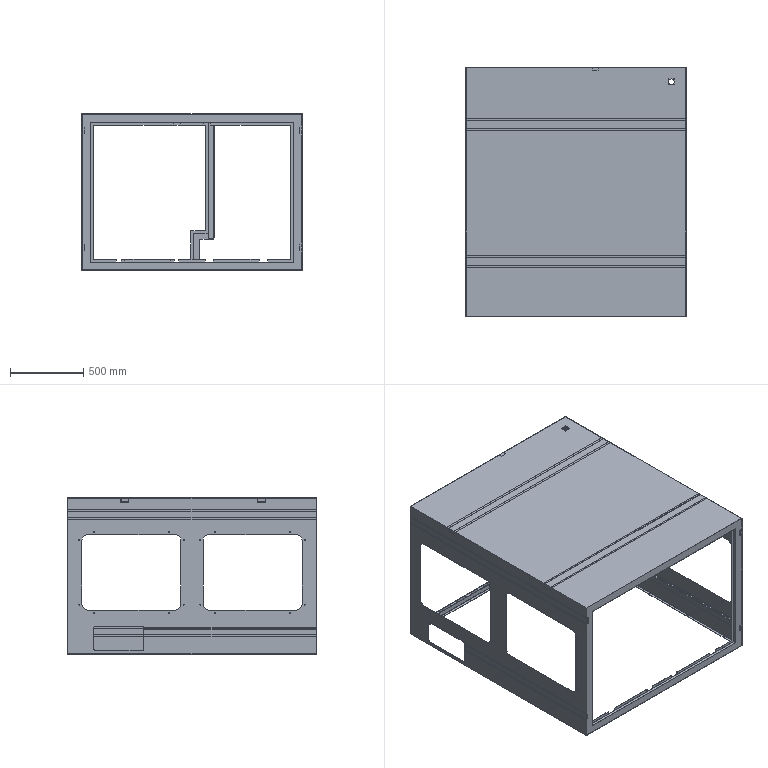Part | STEP file | 11-FG-JX00611 | 5 solids | 618 faces | box 1500 x 1700 x 1065 mm | volume 13737481 mm3 | plane 391 | cylinder 227 | commonest cylinder face diameters 6 x64 3.3 x36 5.5 x23 1.473 x16 2 x16 2.5 x16